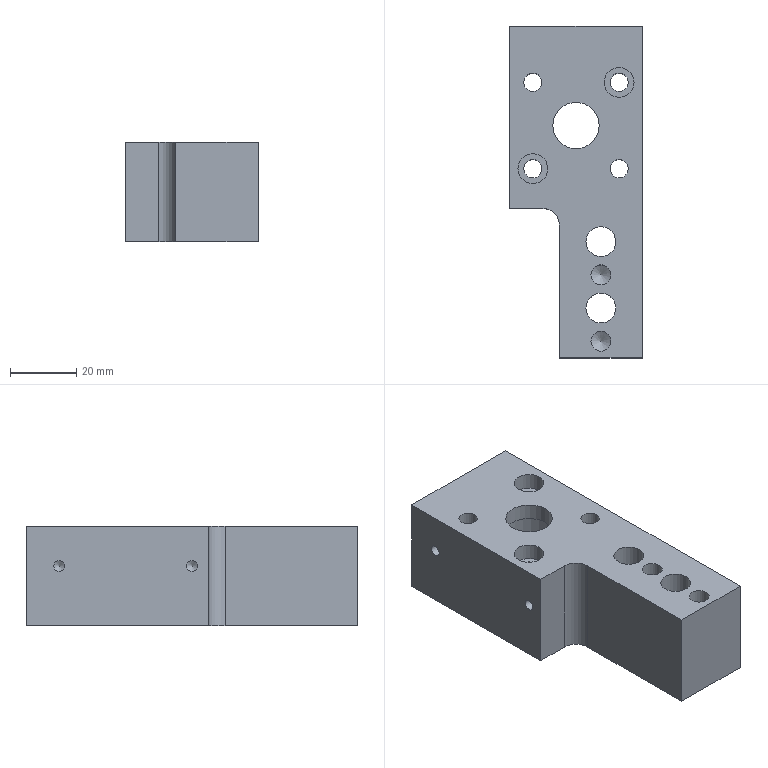Part | NX | features BREP 1 | 1 solid | 50 faces | box 40 x 100 x 30 mm | volume 78075 mm3 | cylinder 25 | plane 17 | cone 8 | commonest cylinder face diameters 10 x5 5.5 x4 6 x4 9 x4 3.3 x2 5 x2
STEP:
#1=CARTESIAN_POINT('',(-15.75,9.5,-9.6));
#2=VERTEX_POINT('',#1);
#3=CARTESIAN_POINT('',(-13.,9.5,-9.6));
#4=DIRECTION('',(0.,0.,-1.));
#5=DIRECTION('',(-1.,0.,0.));
#6=AXIS2_PLACEMENT_3D('',#3,#4,#5);
#7=CIRCLE('',#6,2.75);
#8=EDGE_CURVE('',#2,#2,#7,.T.);
#9=ORIENTED_EDGE('',*,*,#8,.T.);
#10=EDGE_LOOP('',(#9));
#11=FACE_BOUND('',#10,.T.);
#12=CARTESIAN_POINT('',(-10.25,9.5,10.));
#13=VERTEX_POINT('',#12);
#14=CARTESIAN_POINT('',(-13.,9.5,10.));
#15=DIRECTION('',(0.,0.,-1.));
#16=DIRECTION('',(1.,0.,0.));
#17=AXIS2_PLACEMENT_3D('',#14,#15,#16);
#18=CIRCLE('',#17,2.75);
#19=EDGE_CURVE('',#13,#13,#18,.T.);
#20=ORIENTED_EDGE('',*,*,#19,.F.);
#21=EDGE_LOOP('',(#20));
#22=FACE_BOUND('',#21,.T.);
#23=CARTESIAN_POINT('',(-13.,9.5,-15.));
#24=DIRECTION('',(0.,0.,-1.));
#25=DIRECTION('',(1.,0.,0.));
#26=AXIS2_PLACEMENT_3D('',#23,#24,#25);
#27=CYLINDRICAL_SURFACE('',#26,2.75);
#28=ADVANCED_FACE('',(#11,#22),#27,.F.);
#29=CARTESIAN_POINT('',(10.25,35.5,-9.6));
#30=VERTEX_POINT('',#29);
#31=CARTESIAN_POINT('',(13.,35.5,-9.6));
#32=DIRECTION('',(0.,0.,-1.));
#33=DIRECTION('',(-1.,0.,0.));
#34=AXIS2_PLACEMENT_3D('',#31,#32,#33);
#35=CIRCLE('',#34,2.75);
#36=EDGE_CURVE('',#30,#30,#35,.T.);
#37=ORIENTED_EDGE('',*,*,#36,.T.);
#38=EDGE_LOOP('',(#37));
#39=FACE_BOUND('',#38,.T.);
#40=CARTESIAN_POINT('',(15.75,35.5,10.));
#41=VERTEX_POINT('',#40);
#42=CARTESIAN_POINT('',(13.,35.5,10.));
#43=DIRECTION('',(0.,0.,-1.));
#44=DIRECTION('',(1.,0.,0.));
#45=AXIS2_PLACEMENT_3D('',#42,#43,#44);
#46=CIRCLE('',#45,2.75);
#47=EDGE_CURVE('',#41,#41,#46,.T.);
#48=ORIENTED_EDGE('',*,*,#47,.F.);
#49=EDGE_LOOP('',(#48));
#50=FACE_BOUND('',#49,.T.);
#51=CARTESIAN_POINT('',(13.,35.5,-15.));
#52=DIRECTION('',(0.,0.,-1.));
#53=DIRECTION('',(1.,0.,0.));
#54=AXIS2_PLACEMENT_3D('',#51,#52,#53);
#55=CYLINDRICAL_SURFACE('',#54,2.75);
#56=ADVANCED_FACE('',(#39,#50),#55,.F.);
#57=CARTESIAN_POINT('',(-10.5,22.5,-15.));
#58=VERTEX_POINT('',#57);
#59=CARTESIAN_POINT('',(0.,22.5,-15.));
#60=DIRECTION('',(0.,0.,-1.));
#61=DIRECTION('',(-1.,0.,0.));
#62=AXIS2_PLACEMENT_3D('',#59,#60,#61);
#63=CIRCLE('',#62,10.5);
#64=EDGE_CURVE('',#58,#58,#63,.T.);
#65=ORIENTED_EDGE('',*,*,#64,.T.);
#66=EDGE_LOOP('',(#65));
#67=FACE_BOUND('',#66,.T.);
#68=CARTESIAN_POINT('',(10.5,22.5,10.));
#69=VERTEX_POINT('',#68);
#70=CARTESIAN_POINT('',(0.,22.5,10.));
#71=DIRECTION('',(0.,0.,-1.));
#72=DIRECTION('',(1.,0.,0.));
#73=AXIS2_PLACEMENT_3D('',#70,#71,#72);
#74=CIRCLE('',#73,10.5);
#75=EDGE_CURVE('',#69,#69,#74,.T.);
#76=ORIENTED_EDGE('',*,*,#75,.F.);
#77=EDGE_LOOP('',(#76));
#78=FACE_BOUND('',#77,.T.);
#79=CARTESIAN_POINT('',(0.,22.5,-15.));
#80=DIRECTION('',(0.,0.,-1.));
#81=DIRECTION('',(1.,0.,0.));
#82=AXIS2_PLACEMENT_3D('',#79,#80,#81);
#83=CYLINDRICAL_SURFACE('',#82,10.5);
#84=ADVANCED_FACE('',(#67,#78),#83,.F.);
#85=CARTESIAN_POINT('',(20.,-47.5,15.));
#86=VERTEX_POINT('',#85);
#87=CARTESIAN_POINT('',(20.,52.5,15.));
#88=VERTEX_POINT('',#87);
#89=CARTESIAN_POINT('',(20.,-52.5,15.));
#90=DIRECTION('',(0.,1.,0.));
#91=VECTOR('',#90,1000.);
#92=LINE('',#89,#91);
#93=EDGE_CURVE('',#86,#88,#92,.T.);
#94=ORIENTED_EDGE('',*,*,#93,.F.);
#95=CARTESIAN_POINT('',(20.,-47.5,-15.));
#96=VERTEX_POINT('',#95);
#97=CARTESIAN_POINT('',(20.,-47.5,40.495));
#98=DIRECTION('',(0.,0.,-1.));
#99=VECTOR('',#98,1000.);
#100=LINE('',#97,#99);
#101=EDGE_CURVE('',#86,#96,#100,.T.);
#102=ORIENTED_EDGE('',*,*,#101,.T.);
#103=CARTESIAN_POINT('',(20.,52.5,-15.));
#104=VERTEX_POINT('',#103);
#105=CARTESIAN_POINT('',(20.,-52.5,-15.));
#106=DIRECTION('',(0.,1.,0.));
#107=VECTOR('',#106,1000.);
#108=LINE('',#105,#107);
#109=EDGE_CURVE('',#96,#104,#108,.T.);
#110=ORIENTED_EDGE('',*,*,#109,.T.);
#111=CARTESIAN_POINT('',(20.,52.5,15.));
#112=DIRECTION('',(0.,0.,-1.));
#113=VECTOR('',#112,1000.);
#114=LINE('',#111,#113);
#115=EDGE_CURVE('',#88,#104,#114,.T.);
#116=ORIENTED_EDGE('',*,*,#115,.F.);
#117=EDGE_LOOP('',(#94,#102,#110,#116));
#118=FACE_BOUND('',#117,.T.);
#119=CARTESIAN_POINT('',(20.,-52.5,15.));
#120=DIRECTION('',(-1.,0.,0.));
#121=DIRECTION('',(0.,0.,-1.));
#122=AXIS2_PLACEMENT_3D('',#119,#120,#121);
#123=PLANE('',#122);
#124=ADVANCED_FACE('',(#118),#123,.F.);
#125=CARTESIAN_POINT('',(-20.,52.5,-15.));
#126=VERTEX_POINT('',#125);
#127=CARTESIAN_POINT('',(-20.,52.5,-15.));
#128=DIRECTION('',(-1.,0.,0.));
#129=VECTOR('',#128,1000.);
#130=LINE('',#127,#129);
#131=EDGE_CURVE('',#104,#126,#130,.T.);
#132=ORIENTED_EDGE('',*,*,#131,.T.);
#133=CARTESIAN_POINT('',(-20.,52.5,15.));
#134=VERTEX_POINT('',#133);
#135=CARTESIAN_POINT('',(-20.,52.5,15.));
#136=DIRECTION('',(0.,0.,-1.));
#137=VECTOR('',#136,1000.);
#138=LINE('',#135,#137);
#139=EDGE_CURVE('',#134,#126,#138,.T.);
#140=ORIENTED_EDGE('',*,*,#139,.F.);
#141=CARTESIAN_POINT('',(-20.,52.5,15.));
#142=DIRECTION('',(-1.,0.,0.));
#143=VECTOR('',#142,1000.);
#144=LINE('',#141,#143);
#145=EDGE_CURVE('',#88,#134,#144,.T.);
#146=ORIENTED_EDGE('',*,*,#145,.F.);
#147=ORIENTED_EDGE('',*,*,#115,.T.);
#148=EDGE_LOOP('',(#132,#140,#146,#147));
#149=FACE_BOUND('',#148,.T.);
#150=CARTESIAN_POINT('',(-20.,52.5,15.));
#151=DIRECTION('',(0.,-1.,0.));
#152=DIRECTION('',(0.,0.,1.));
#153=AXIS2_PLACEMENT_3D('',#150,#151,#152);
#154=PLANE('',#153);
#155=ADVANCED_FACE('',(#149),#154,.F.);
#156=CARTESIAN_POINT('',(-20.,42.5,4.65));
#157=VERTEX_POINT('',#156);
#158=CARTESIAN_POINT('',(-20.,42.5,3.));
#159=DIRECTION('',(-1.,0.,0.));
#160=DIRECTION('',(0.,0.,1.));
#161=AXIS2_PLACEMENT_3D('',#158,#159,#160);
#162=CIRCLE('',#161,1.65);
#163=EDGE_CURVE('',#157,#157,#162,.T.);
#164=ORIENTED_EDGE('',*,*,#163,.F.);
#165=EDGE_LOOP('',(#164));
#166=FACE_BOUND('',#165,.T.);
#167=CARTESIAN_POINT('',(-20.,2.5,4.65));
#168=VERTEX_POINT('',#167);
#169=CARTESIAN_POINT('',(-20.,2.5,3.));
#170=DIRECTION('',(-1.,0.,0.));
#171=DIRECTION('',(0.,0.,1.));
#172=AXIS2_PLACEMENT_3D('',#169,#170,#171);
#173=CIRCLE('',#172,1.65);
#174=EDGE_CURVE('',#168,#168,#173,.T.);
#175=ORIENTED_EDGE('',*,*,#174,.F.);
#176=EDGE_LOOP('',(#175));
#177=FACE_BOUND('',#176,.T.);
#178=CARTESIAN_POINT('',(-20.,-2.5,-15.));
#179=VERTEX_POINT('',#178);
#180=CARTESIAN_POINT('',(-20.,-52.5,-15.));
#181=DIRECTION('',(0.,-1.,0.));
#182=VECTOR('',#181,1000.);
#183=LINE('',#180,#182);
#184=EDGE_CURVE('',#126,#179,#183,.T.);
#185=ORIENTED_EDGE('',*,*,#184,.T.);
#186=CARTESIAN_POINT('',(-20.,-2.5,15.));
#187=VERTEX_POINT('',#186);
#188=CARTESIAN_POINT('',(-20.,-2.5,67.202));
#189=DIRECTION('',(0.,0.,-1.));
#190=VECTOR('',#189,1000.);
#191=LINE('',#188,#190);
#192=EDGE_CURVE('',#187,#179,#191,.T.);
#193=ORIENTED_EDGE('',*,*,#192,.F.);
#194=CARTESIAN_POINT('',(-20.,-52.5,15.));
#195=DIRECTION('',(0.,-1.,0.));
#196=VECTOR('',#195,1000.);
#197=LINE('',#194,#196);
#198=EDGE_CURVE('',#134,#187,#197,.T.);
#199=ORIENTED_EDGE('',*,*,#198,.F.);
#200=ORIENTED_EDGE('',*,*,#139,.T.);
#201=EDGE_LOOP('',(#185,#193,#199,#200));
#202=FACE_BOUND('',#201,.T.);
#203=CARTESIAN_POINT('',(-20.,-52.5,15.));
#204=DIRECTION('',(1.,0.,0.));
#205=DIRECTION('',(0.,0.,1.));
#206=AXIS2_PLACEMENT_3D('',#203,#204,#205);
#207=PLANE('',#206);
#208=ADVANCED_FACE('',(#166,#177,#202),#207,.F.);
#209=CARTESIAN_POINT('',(17.5,35.5,15.));
#210=VERTEX_POINT('',#209);
#211=CARTESIAN_POINT('',(13.,35.5,15.));
#212=DIRECTION('',(0.,0.,1.));
#213=DIRECTION('',(1.,0.,0.));
#214=AXIS2_PLACEMENT_3D('',#211,#212,#213);
#215=CIRCLE('',#214,4.5);
#216=EDGE_CURVE('',#210,#210,#215,.T.);
#217=ORIENTED_EDGE('',*,*,#216,.F.);
#218=EDGE_LOOP('',(#217));
#219=FACE_BOUND('',#218,.T.);
#220=CARTESIAN_POINT('',(-8.5,9.5,15.));
#221=VERTEX_POINT('',#220);
#222=CARTESIAN_POINT('',(-13.,9.5,15.));
#223=DIRECTION('',(0.,0.,1.));
#224=DIRECTION('',(1.,0.,0.));
#225=AXIS2_PLACEMENT_3D('',#222,#223,#224);
#226=CIRCLE('',#225,4.5);
#227=EDGE_CURVE('',#221,#221,#226,.T.);
#228=ORIENTED_EDGE('',*,*,#227,.F.);
#229=EDGE_LOOP('',(#228));
#230=FACE_BOUND('',#229,.T.);
#231=CARTESIAN_POINT('',(10.25,9.5,15.));
#232=VERTEX_POINT('',#231);
#233=CARTESIAN_POINT('',(13.,9.5,15.));
#234=DIRECTION('',(0.,0.,-1.));
#235=DIRECTION('',(-1.,0.,0.));
#236=AXIS2_PLACEMENT_3D('',#233,#234,#235);
#237=CIRCLE('',#236,2.75);
#238=EDGE_CURVE('',#232,#232,#237,.T.);
#239=ORIENTED_EDGE('',*,*,#238,.T.);
#240=EDGE_LOOP('',(#239));
#241=FACE_BOUND('',#240,.T.);
#242=CARTESIAN_POINT('',(-15.75,35.5,15.));
#243=VERTEX_POINT('',#242);
#244=CARTESIAN_POINT('',(-13.,35.5,15.));
#245=DIRECTION('',(0.,0.,-1.));
#246=DIRECTION('',(-1.,0.,0.));
#247=AXIS2_PLACEMENT_3D('',#244,#245,#246);
#248=CIRCLE('',#247,2.75);
#249=EDGE_CURVE('',#243,#243,#248,.T.);
#250=ORIENTED_EDGE('',*,*,#249,.T.);
#251=EDGE_LOOP('',(#250));
#252=FACE_BOUND('',#251,.T.);
#253=CARTESIAN_POINT('',(3.,-12.5,15.));
#254=VERTEX_POINT('',#253);
#255=CARTESIAN_POINT('',(7.5,-12.5,15.));
#256=DIRECTION('',(0.,0.,-1.));
#257=DIRECTION('',(-1.,0.,0.));
#258=AXIS2_PLACEMENT_3D('',#255,#256,#257);
#259=CIRCLE('',#258,4.5);
#260=EDGE_CURVE('',#254,#254,#259,.T.);
#261=ORIENTED_EDGE('',*,*,#260,.T.);
#262=EDGE_LOOP('',(#261));
#263=FACE_BOUND('',#262,.T.);
#264=CARTESIAN_POINT('',(3.,-32.5,15.));
#265=VERTEX_POINT('',#264);
#266=CARTESIAN_POINT('',(7.5,-32.5,15.));
#267=DIRECTION('',(0.,0.,-1.));
#268=DIRECTION('',(-1.,0.,0.));
#269=AXIS2_PLACEMENT_3D('',#266,#267,#268);
#270=CIRCLE('',#269,4.5);
#271=EDGE_CURVE('',#265,#265,#270,.T.);
#272=ORIENTED_EDGE('',*,*,#271,.T.);
#273=EDGE_LOOP('',(#272));
#274=FACE_BOUND('',#273,.T.);
#275=CARTESIAN_POINT('',(10.5,-42.5,15.));
#276=VERTEX_POINT('',#275);
#277=CARTESIAN_POINT('',(7.5,-42.5,15.));
#278=DIRECTION('',(0.,0.,1.));
#279=DIRECTION('',(1.,0.,0.));
#280=AXIS2_PLACEMENT_3D('',#277,#278,#279);
#281=CIRCLE('',#280,3.);
#282=EDGE_CURVE('',#276,#276,#281,.T.);
#283=ORIENTED_EDGE('',*,*,#282,.F.);
#284=EDGE_LOOP('',(#283));
#285=FACE_BOUND('',#284,.T.);
#286=CARTESIAN_POINT('',(10.5,-22.5,15.));
#287=VERTEX_POINT('',#286);
#288=CARTESIAN_POINT('',(7.5,-22.5,15.));
#289=DIRECTION('',(0.,0.,1.));
#290=DIRECTION('',(1.,0.,0.));
#291=AXIS2_PLACEMENT_3D('',#288,#289,#290);
#292=CIRCLE('',#291,3.);
#293=EDGE_CURVE('',#287,#287,#292,.T.);
#294=ORIENTED_EDGE('',*,*,#293,.F.);
#295=EDGE_LOOP('',(#294));
#296=FACE_BOUND('',#295,.T.);
#297=CARTESIAN_POINT('',(-5.,-47.5,15.));
#298=VERTEX_POINT('',#297);
#299=CARTESIAN_POINT('',(-5.,-7.5,15.));
#300=VERTEX_POINT('',#299);
#301=CARTESIAN_POINT('',(-5.,-2.5,15.));
#302=DIRECTION('',(0.,1.,0.));
#303=VECTOR('',#302,1000.);
#304=LINE('',#301,#303);
#305=EDGE_CURVE('',#298,#300,#304,.T.);
#306=ORIENTED_EDGE('',*,*,#305,.F.);
#307=CARTESIAN_POINT('',(-5.,-47.5,15.));
#308=DIRECTION('',(-1.,0.,0.));
#309=VECTOR('',#308,1000.);
#310=LINE('',#307,#309);
#311=EDGE_CURVE('',#86,#298,#310,.T.);
#312=ORIENTED_EDGE('',*,*,#311,.F.);
#313=ORIENTED_EDGE('',*,*,#93,.T.);
#314=ORIENTED_EDGE('',*,*,#145,.T.);
#315=ORIENTED_EDGE('',*,*,#198,.T.);
#316=CARTESIAN_POINT('',(-10.,-2.5,15.));
#317=VERTEX_POINT('',#316);
#318=CARTESIAN_POINT('',(-20.,-2.5,15.));
#319=DIRECTION('',(-1.,0.,0.));
#320=VECTOR('',#319,1000.);
#321=LINE('',#318,#320);
#322=EDGE_CURVE('',#317,#187,#321,.T.);
#323=ORIENTED_EDGE('',*,*,#322,.F.);
#324=CARTESIAN_POINT('',(-10.,-7.5,15.));
#325=DIRECTION('',(0.,0.,-1.));
#326=DIRECTION('',(-1.,0.,0.));
#327=AXIS2_PLACEMENT_3D('',#324,#325,#326);
#328=CIRCLE('',#327,5.);
#329=EDGE_CURVE('',#317,#300,#328,.T.);
#330=ORIENTED_EDGE('',*,*,#329,.T.);
#331=EDGE_LOOP('',(#306,#312,#313,#314,#315,#323,#330));
#332=FACE_BOUND('',#331,.T.);
#333=CARTESIAN_POINT('',(7.,22.5,15.));
#334=VERTEX_POINT('',#333);
#335=CARTESIAN_POINT('',(0.,22.5,15.));
#336=DIRECTION('',(0.,0.,1.));
#337=DIRECTION('',(1.,0.,0.));
#338=AXIS2_PLACEMENT_3D('',#335,#336,#337);
#339=CIRCLE('',#338,7.);
#340=EDGE_CURVE('',#334,#334,#339,.T.);
#341=ORIENTED_EDGE('',*,*,#340,.F.);
#342=EDGE_LOOP('',(#341));
#343=FACE_BOUND('',#342,.T.);
#344=CARTESIAN_POINT('',(0.,0.,15.));
#345=DIRECTION('',(0.,0.,-1.));
#346=DIRECTION('',(1.,0.,0.));
#347=AXIS2_PLACEMENT_3D('',#344,#345,#346);
#348=PLANE('',#347);
#349=ADVANCED_FACE('',(#219,#230,#241,#252,#263,#274,#285,#296,#332,#343),#348,.F.);
#350=CARTESIAN_POINT('',(-5.,-47.5,-15.));
#351=VERTEX_POINT('',#350);
#352=CARTESIAN_POINT('',(-5.,-47.5,-15.));
#353=DIRECTION('',(1.,0.,0.));
#354=VECTOR('',#353,1000.);
#355=LINE('',#352,#354);
#356=EDGE_CURVE('',#351,#96,#355,.T.);
#357=ORIENTED_EDGE('',*,*,#356,.F.);
#358=CARTESIAN_POINT('',(-5.,-7.5,-15.));
#359=VERTEX_POINT('',#358);
#360=CARTESIAN_POINT('',(-5.,-2.5,-15.));
#361=DIRECTION('',(0.,-1.,0.));
#362=VECTOR('',#361,1000.);
#363=LINE('',#360,#362);
#364=EDGE_CURVE('',#359,#351,#363,.T.);
#365=ORIENTED_EDGE('',*,*,#364,.F.);
#366=CARTESIAN_POINT('',(-10.,-2.5,-15.));
#367=VERTEX_POINT('',#366);
#368=CARTESIAN_POINT('',(-10.,-7.5,-15.));
#369=DIRECTION('',(0.,0.,1.));
#370=DIRECTION('',(-1.,0.,0.));
#371=AXIS2_PLACEMENT_3D('',#368,#369,#370);
#372=CIRCLE('',#371,5.);
#373=EDGE_CURVE('',#359,#367,#372,.T.);
#374=ORIENTED_EDGE('',*,*,#373,.T.);
#375=CARTESIAN_POINT('',(-20.,-2.5,-15.));
#376=DIRECTION('',(1.,0.,0.));
#377=VECTOR('',#376,1000.);
#378=LINE('',#375,#377);
#379=EDGE_CURVE('',#179,#367,#378,.T.);
#380=ORIENTED_EDGE('',*,*,#379,.F.);
#381=ORIENTED_EDGE('',*,*,#184,.F.);
#382=ORIENTED_EDGE('',*,*,#131,.F.);
#383=ORIENTED_EDGE('',*,*,#109,.F.);
#384=EDGE_LOOP('',(#357,#365,#374,#380,#381,#382,#383));
#385=FACE_BOUND('',#384,.T.);
#386=CARTESIAN_POINT('',(-13.,45.,-15.));
#387=VERTEX_POINT('',#386);
#388=CARTESIAN_POINT('',(-10.,45.,-15.));
#389=DIRECTION('',(0.,0.,-1.));
#390=DIRECTION('',(-1.,0.,0.));
#391=AXIS2_PLACEMENT_3D('',#388,#389,#390);
#392=CIRCLE('',#391,3.);
#393=EDGE_CURVE('',#387,#387,#392,.T.);
#394=ORIENTED_EDGE('',*,*,#393,.F.);
#395=EDGE_LOOP('',(#394));
#396=FACE_BOUND('',#395,.T.);
#397=CARTESIAN_POINT('',(7.,0.,-15.));
#398=VERTEX_POINT('',#397);
#399=CARTESIAN_POINT('',(10.,0.,-15.));
#400=DIRECTION('',(0.,0.,-1.));
#401=DIRECTION('',(-1.,0.,0.));
#402=AXIS2_PLACEMENT_3D('',#399,#400,#401);
#403=CIRCLE('',#402,3.);
#404=EDGE_CURVE('',#398,#398,#403,.T.);
#405=ORIENTED_EDGE('',*,*,#404,.F.);
#406=EDGE_LOOP('',(#405));
#407=FACE_BOUND('',#406,.T.);
#408=CARTESIAN_POINT('',(-2.5,45.,-15.));
#409=VERTEX_POINT('',#408);
#410=CARTESIAN_POINT('',(0.,45.,-15.));
#411=DIRECTION('',(0.,0.,-1.));
#412=DIRECTION('',(-1.,0.,0.));
#413=AXIS2_PLACEMENT_3D('',#410,#411,#412);
#414=CIRCLE('',#413,2.5);
#415=EDGE_CURVE('',#409,#409,#414,.T.);
#416=ORIENTED_EDGE('',*,*,#415,.F.);
#417=EDGE_LOOP('',(#416));
#418=FACE_BOUND('',#417,.T.);
#419=CARTESIAN_POINT('',(-2.5,0.,-15.));
#420=VERTEX_POINT('',#419);
#421=CARTESIAN_POINT('',(0.,0.,-15.));
#422=DIRECTION('',(0.,0.,-1.));
#423=DIRECTION('',(-1.,0.,0.));
#424=AXIS2_PLACEMENT_3D('',#421,#422,#423);
#425=CIRCLE('',#424,2.5);
#426=EDGE_CURVE('',#420,#420,#425,.T.);
#427=ORIENTED_EDGE('',*,*,#426,.F.);
#428=EDGE_LOOP('',(#427));
#429=FACE_BOUND('',#428,.T.);
#430=CARTESIAN_POINT('',(8.,35.5,-15.));
#431=VERTEX_POINT('',#430);
#432=CARTESIAN_POINT('',(13.,35.5,-15.));
#433=DIRECTION('',(0.,0.,-1.));
#434=DIRECTION('',(-1.,0.,0.));
#435=AXIS2_PLACEMENT_3D('',#432,#433,#434);
#436=CIRCLE('',#435,5.);
#437=EDGE_CURVE('',#431,#431,#436,.T.);
#438=ORIENTED_EDGE('',*,*,#437,.F.);
#439=EDGE_LOOP('',(#438));
#440=FACE_BOUND('',#439,.T.);
#441=CARTESIAN_POINT('',(-18.,9.5,-15.));
#442=VERTEX_POINT('',#441);
#443=CARTESIAN_POINT('',(-13.,9.5,-15.));
#444=DIRECTION('',(0.,0.,-1.));
#445=DIRECTION('',(-1.,0.,0.));
#446=AXIS2_PLACEMENT_3D('',#443,#444,#445);
#447=CIRCLE('',#446,5.);
#448=EDGE_CURVE('',#442,#442,#447,.T.);
#449=ORIENTED_EDGE('',*,*,#448,.F.);
#450=EDGE_LOOP('',(#449));
#451=FACE_BOUND('',#450,.T.);
#452=CARTESIAN_POINT('',(8.,9.5,-15.));
#453=VERTEX_POINT('',#452);
#454=CARTESIAN_POINT('',(13.,9.5,-15.));
#455=DIRECTION('',(0.,0.,-1.));
#456=DIRECTION('',(-1.,0.,0.));
#457=AXIS2_PLACEMENT_3D('',#454,#455,#456);
#458=CIRCLE('',#457,5.);
#459=EDGE_CURVE('',#453,#453,#458,.T.);
#460=ORIENTED_EDGE('',*,*,#459,.F.);
#461=EDGE_LOOP('',(#460));
#462=FACE_BOUND('',#461,.T.);
#463=CARTESIAN_POINT('',(-18.,35.5,-15.));
#464=VERTEX_POINT('',#463);
#465=CARTESIAN_POINT('',(-13.,35.5,-15.));
#466=DIRECTION('',(0.,0.,-1.));
#467=DIRECTION('',(-1.,0.,0.));
#468=AXIS2_PLACEMENT_3D('',#465,#466,#467);
#469=CIRCLE('',#468,5.);
#470=EDGE_CURVE('',#464,#464,#469,.T.);
#471=ORIENTED_EDGE('',*,*,#470,.F.);
#472=EDGE_LOOP('',(#471));
#473=FACE_BOUND('',#472,.T.);
#474=CARTESIAN_POINT('',(0.,-12.5,-15.));
#475=VERTEX_POINT('',#474);
#476=CARTESIAN_POINT('',(7.5,-12.5,-15.));
#477=DIRECTION('',(0.,0.,-1.));
#478=DIRECTION('',(-1.,0.,0.));
#479=AXIS2_PLACEMENT_3D('',#476,#477,#478);
#480=CIRCLE('',#479,7.5);
#481=EDGE_CURVE('',#475,#475,#480,.T.);
#482=ORIENTED_EDGE('',*,*,#481,.F.);
#483=EDGE_LOOP('',(#482));
#484=FACE_BOUND('',#483,.T.);
#485=CARTESIAN_POINT('',(0.,-32.5,-15.));
#486=VERTEX_POINT('',#485);
#487=CARTESIAN_POINT('',(7.5,-32.5,-15.));
#488=DIRECTION('',(0.,0.,-1.));
#489=DIRECTION('',(-1.,0.,0.));
#490=AXIS2_PLACEMENT_3D('',#487,#488,#489);
#491=CIRCLE('',#490,7.5);
#492=EDGE_CURVE('',#486,#486,#491,.T.);
#493=ORIENTED_EDGE('',*,*,#492,.F.);
#494=EDGE_LOOP('',(#493));
#495=FACE_BOUND('',#494,.T.);
#496=ORIENTED_EDGE('',*,*,#64,.F.);
#497=EDGE_LOOP('',(#496));
#498=FACE_BOUND('',#497,.T.);
#499=CARTESIAN_POINT('',(0.,0.,-15.));
#500=DIRECTION('',(0.,0.,-1.));
#501=DIRECTION('',(1.,0.,0.));
#502=AXIS2_PLACEMENT_3D('',#499,#500,#501);
#503=PLANE('',#502);
#504=ADVANCED_FACE('',(#385,#396,#407,#418,#429,#440,#451,#462,#473,#484,#495,#498),#503,.T.);
#505=CARTESIAN_POINT('',(7.,22.5,10.));
#506=VERTEX_POINT('',#505);
#507=CARTESIAN_POINT('',(0.,22.5,10.));
#508=DIRECTION('',(0.,0.,1.));
#509=DIRECTION('',(1.,0.,0.));
#510=AXIS2_PLACEMENT_3D('',#507,#508,#509);
#511=CIRCLE('',#510,7.);
#512=EDGE_CURVE('',#506,#506,#511,.T.);
#513=ORIENTED_EDGE('',*,*,#512,.T.);
#514=EDGE_LOOP('',(#513));
#515=FACE_BOUND('',#514,.T.);
#516=ORIENTED_EDGE('',*,*,#75,.T.);
#517=EDGE_LOOP('',(#516));
#518=FACE_BOUND('',#517,.T.);
#519=CARTESIAN_POINT('',(0.,22.5,10.));
#520=DIRECTION('',(0.,0.,1.));
#521=DIRECTION('',(-1.,0.,0.));
#522=AXIS2_PLACEMENT_3D('',#519,#520,#521);
#523=PLANE('',#522);
#524=ADVANCED_FACE('',(#515,#518),#523,.F.);
#525=ORIENTED_EDGE('',*,*,#512,.F.);
#526=EDGE_LOOP('',(#525));
#527=FACE_BOUND('',#526,.T.);
#528=ORIENTED_EDGE('',*,*,#340,.T.);
#529=EDGE_LOOP('',(#528));
#530=FACE_BOUND('',#529,.T.);
#531=CARTESIAN_POINT('',(0.,22.5,10.));
#532=DIRECTION('',(0.,0.,1.));
#533=DIRECTION('',(-1.,0.,0.));
#534=AXIS2_PLACEMENT_3D('',#531,#532,#533);
#535=CYLINDRICAL_SURFACE('',#534,7.);
#536=ADVANCED_FACE('',(#527,#530),#535,.F.);
#537=ORIENTED_EDGE('',*,*,#364,.T.);
#538=CARTESIAN_POINT('',(-5.,-47.5,40.495));
#539=DIRECTION('',(0.,0.,-1.));
#540=VECTOR('',#539,1000.);
#541=LINE('',#538,#540);
#542=EDGE_CURVE('',#298,#351,#541,.T.);
#543=ORIENTED_EDGE('',*,*,#542,.F.);
#544=ORIENTED_EDGE('',*,*,#305,.T.);
#545=CARTESIAN_POINT('',(-5.,-7.5,-15.));
#546=DIRECTION('',(0.,0.,-1.));
#547=VECTOR('',#546,1000.);
#548=LINE('',#545,#547);
#549=EDGE_CURVE('',#300,#359,#548,.T.);
#550=ORIENTED_EDGE('',*,*,#549,.T.);
#551=EDGE_LOOP('',(#537,#543,#544,#550));
#552=FACE_BOUND('',#551,.T.);
#553=CARTESIAN_POINT('',(-5.,-2.5,67.202));
#554=DIRECTION('',(1.,0.,0.));
#555=DIRECTION('',(0.,-1.,0.));
#556=AXIS2_PLACEMENT_3D('',#553,#554,#555);
#557=PLANE('',#556);
#558=ADVANCED_FACE('',(#552),#557,.F.);
#559=ORIENTED_EDGE('',*,*,#379,.T.);
#560=CARTESIAN_POINT('',(-10.,-2.5,15.));
#561=DIRECTION('',(0.,0.,1.));
#562=VECTOR('',#561,1000.);
#563=LINE('',#560,#562);
#564=EDGE_CURVE('',#367,#317,#563,.T.);
#565=ORIENTED_EDGE('',*,*,#564,.T.);
#566=ORIENTED_EDGE('',*,*,#322,.T.);
#567=ORIENTED_EDGE('',*,*,#192,.T.);
#568=EDGE_LOOP('',(#559,#565,#566,#567));
#569=FACE_BOUND('',#568,.T.);
#570=CARTESIAN_POINT('',(-20.,-2.5,67.202));
#571=DIRECTION('',(0.,1.,0.));
#572=DIRECTION('',(0.,0.,-1.));
#573=AXIS2_PLACEMENT_3D('',#570,#571,#572);
#574=PLANE('',#573);
#575=ADVANCED_FACE('',(#569),#574,.F.);
#576=CARTESIAN_POINT('',(7.5,-22.5,1.197));
#577=VERTEX_POINT('',#576);
#578=VERTEX_LOOP('',#577);
#579=FACE_BOUND('',#578,.T.);
#580=CARTESIAN_POINT('',(10.5,-22.5,3.));
#581=VERTEX_POINT('',#580);
#582=CARTESIAN_POINT('',(7.5,-22.5,3.));
#583=DIRECTION('',(0.,0.,1.));
#584=DIRECTION('',(1.,0.,0.));
#585=AXIS2_PLACEMENT_3D('',#582,#583,#584);
#586=CIRCLE('',#585,3.);
#587=EDGE_CURVE('',#581,#581,#586,.T.);
#588=ORIENTED_EDGE('',*,*,#587,.T.);
#589=EDGE_LOOP('',(#588));
#590=FACE_BOUND('',#589,.T.);
#591=CARTESIAN_POINT('',(7.5,-22.5,3.));
#592=DIRECTION('',(0.,0.,1.));
#593=DIRECTION('',(-1.,0.,0.));
#594=AXIS2_PLACEMENT_3D('',#591,#592,#593);
#595=CONICAL_SURFACE('',#594,3.,1.03);
#596=ADVANCED_FACE('',(#579,#590),#595,.F.);
#597=ORIENTED_EDGE('',*,*,#587,.F.);
#598=EDGE_LOOP('',(#597));
#599=FACE_BOUND('',#598,.T.);
#600=ORIENTED_EDGE('',*,*,#293,.T.);
#601=EDGE_LOOP('',(#600));
#602=FACE_BOUND('',#601,.T.);
#603=CARTESIAN_POINT('',(7.5,-22.5,15.));
#604=DIRECTION('',(0.,0.,1.));
#605=DIRECTION('',(-1.,0.,0.));
#606=AXIS2_PLACEMENT_3D('',#603,#604,#605);
#607=CYLINDRICAL_SURFACE('',#606,3.);
#608=ADVANCED_FACE('',(#599,#602),#607,.F.);
#609=CARTESIAN_POINT('',(7.5,-42.5,1.197));
#610=VERTEX_POINT('',#609);
#611=VERTEX_LOOP('',#610);
#612=FACE_BOUND('',#611,.T.);
#613=CARTESIAN_POINT('',(10.5,-42.5,3.));
#614=VERTEX_POINT('',#613);
#615=CARTESIAN_POINT('',(7.5,-42.5,3.));
#616=DIRECTION('',(0.,0.,1.));
#617=DIRECTION('',(1.,0.,0.));
#618=AXIS2_PLACEMENT_3D('',#615,#616,#617);
#619=CIRCLE('',#618,3.);
#620=EDGE_CURVE('',#614,#614,#619,.T.);
#621=ORIENTED_EDGE('',*,*,#620,.T.);
#622=EDGE_LOOP('',(#621));
#623=FACE_BOUND('',#622,.T.);
#624=CARTESIAN_POINT('',(7.5,-42.5,3.));
#625=DIRECTION('',(0.,0.,1.));
#626=DIRECTION('',(-1.,0.,0.));
#627=AXIS2_PLACEMENT_3D('',#624,#625,#626);
#628=CONICAL_SURFACE('',#627,3.,1.03);
#629=ADVANCED_FACE('',(#612,#623),#628,.F.);
#630=ORIENTED_EDGE('',*,*,#620,.F.);
#631=EDGE_LOOP('',(#630));
#632=FACE_BOUND('',#631,.T.);
#633=ORIENTED_EDGE('',*,*,#282,.T.);
#634=EDGE_LOOP('',(#633));
#635=FACE_BOUND('',#634,.T.);
#636=CARTESIAN_POINT('',(7.5,-42.5,15.));
#637=DIRECTION('',(0.,0.,1.));
#638=DIRECTION('',(-1.,0.,0.));
#639=AXIS2_PLACEMENT_3D('',#636,#637,#638);
#640=CYLINDRICAL_SURFACE('',#639,3.);
#641=ADVANCED_FACE('',(#632,#635),#640,.F.);
#642=ORIENTED_EDGE('',*,*,#271,.F.);
#643=EDGE_LOOP('',(#642));
#644=FACE_BOUND('',#643,.T.);
#645=CARTESIAN_POINT('',(3.,-32.5,-6.4));
#646=VERTEX_POINT('',#645);
#647=CARTESIAN_POINT('',(7.5,-32.5,-6.4));
#648=DIRECTION('',(0.,0.,-1.));
#649=DIRECTION('',(-1.,0.,0.));
#650=AXIS2_PLACEMENT_3D('',#647,#648,#649);
#651=CIRCLE('',#650,4.5);
#652=EDGE_CURVE('',#646,#646,#651,.T.);
#653=ORIENTED_EDGE('',*,*,#652,.T.);
#654=EDGE_LOOP('',(#653));
#655=FACE_BOUND('',#654,.T.);
#656=CARTESIAN_POINT('',(7.5,-32.5,-15.));
#657=DIRECTION('',(0.,0.,-1.));
#658=DIRECTION('',(1.,0.,0.));
#659=AXIS2_PLACEMENT_3D('',#656,#657,#658);
#660=CYLINDRICAL_SURFACE('',#659,4.5);
#661=ADVANCED_FACE('',(#644,#655),#660,.F.);
#662=ORIENTED_EDGE('',*,*,#652,.F.);
#663=EDGE_LOOP('',(#662));
#664=FACE_BOUND('',#663,.T.);
#665=CARTESIAN_POINT('',(0.,-32.5,-6.4));
#666=VERTEX_POINT('',#665);
#667=CARTESIAN_POINT('',(7.5,-32.5,-6.4));
#668=DIRECTION('',(0.,0.,-1.));
#669=DIRECTION('',(-1.,0.,0.));
#670=AXIS2_PLACEMENT_3D('',#667,#668,#669);
#671=CIRCLE('',#670,7.5);
#672=EDGE_CURVE('',#666,#666,#671,.T.);
#673=ORIENTED_EDGE('',*,*,#672,.T.);
#674=EDGE_LOOP('',(#673));
#675=FACE_BOUND('',#674,.T.);
#676=CARTESIAN_POINT('',(12.,-32.5,-6.4));
#677=DIRECTION('',(0.,0.,1.));
#678=DIRECTION('',(-1.,0.,0.));
#679=AXIS2_PLACEMENT_3D('',#676,#677,#678);
#680=PLANE('',#679);
#681=ADVANCED_FACE('',(#664,#675),#680,.F.);
#682=ORIENTED_EDGE('',*,*,#672,.F.);
#683=EDGE_LOOP('',(#682));
#684=FACE_BOUND('',#683,.T.);
#685=ORIENTED_EDGE('',*,*,#492,.T.);
#686=EDGE_LOOP('',(#685));
#687=FACE_BOUND('',#686,.T.);
#688=CARTESIAN_POINT('',(7.5,-32.5,-15.));
#689=DIRECTION('',(0.,0.,-1.));
#690=DIRECTION('',(1.,0.,0.));
#691=AXIS2_PLACEMENT_3D('',#688,#689,#690);
#692=CYLINDRICAL_SURFACE('',#691,7.5);
#693=ADVANCED_FACE('',(#684,#687),#692,.F.);
#694=ORIENTED_EDGE('',*,*,#260,.F.);
#695=EDGE_LOOP('',(#694));
#696=FACE_BOUND('',#695,.T.);
#697=CARTESIAN_POINT('',(3.,-12.5,-6.4));
#698=VERTEX_POINT('',#697);
#699=CARTESIAN_POINT('',(7.5,-12.5,-6.4));
#700=DIRECTION('',(0.,0.,-1.));
#701=DIRECTION('',(-1.,0.,0.));
#702=AXIS2_PLACEMENT_3D('',#699,#700,#701);
#703=CIRCLE('',#702,4.5);
#704=EDGE_CURVE('',#698,#698,#703,.T.);
#705=ORIENTED_EDGE('',*,*,#704,.T.);
#706=EDGE_LOOP('',(#705));
#707=FACE_BOUND('',#706,.T.);
#708=CARTESIAN_POINT('',(7.5,-12.5,-15.));
#709=DIRECTION('',(0.,0.,-1.));
#710=DIRECTION('',(1.,0.,0.));
#711=AXIS2_PLACEMENT_3D('',#708,#709,#710);
#712=CYLINDRICAL_SURFACE('',#711,4.5);
#713=ADVANCED_FACE('',(#696,#707),#712,.F.);
#714=ORIENTED_EDGE('',*,*,#704,.F.);
#715=EDGE_LOOP('',(#714));
#716=FACE_BOUND('',#715,.T.);
#717=CARTESIAN_POINT('',(0.,-12.5,-6.4));
#718=VERTEX_POINT('',#717);
#719=CARTESIAN_POINT('',(7.5,-12.5,-6.4));
#720=DIRECTION('',(0.,0.,-1.));
#721=DIRECTION('',(-1.,0.,0.));
#722=AXIS2_PLACEMENT_3D('',#719,#720,#721);
#723=CIRCLE('',#722,7.5);
#724=EDGE_CURVE('',#718,#718,#723,.T.);
#725=ORIENTED_EDGE('',*,*,#724,.T.);
#726=EDGE_LOOP('',(#725));
#727=FACE_BOUND('',#726,.T.);
#728=CARTESIAN_POINT('',(12.,-12.5,-6.4));
#729=DIRECTION('',(0.,0.,1.));
#730=DIRECTION('',(-1.,0.,0.));
#731=AXIS2_PLACEMENT_3D('',#728,#729,#730);
#732=PLANE('',#731);
#733=ADVANCED_FACE('',(#716,#727),#732,.F.);
#734=ORIENTED_EDGE('',*,*,#724,.F.);
#735=EDGE_LOOP('',(#734));
#736=FACE_BOUND('',#735,.T.);
#737=ORIENTED_EDGE('',*,*,#481,.T.);
#738=EDGE_LOOP('',(#737));
#739=FACE_BOUND('',#738,.T.);
#740=CARTESIAN_POINT('',(7.5,-12.5,-15.));
#741=DIRECTION('',(0.,0.,-1.));
#742=DIRECTION('',(1.,0.,0.));
#743=AXIS2_PLACEMENT_3D('',#740,#741,#742);
#744=CYLINDRICAL_SURFACE('',#743,7.5);
#745=ADVANCED_FACE('',(#736,#739),#744,.F.);
#746=ORIENTED_EDGE('',*,*,#329,.F.);
#747=ORIENTED_EDGE('',*,*,#564,.F.);
#748=ORIENTED_EDGE('',*,*,#373,.F.);
#749=ORIENTED_EDGE('',*,*,#549,.F.);
#750=EDGE_LOOP('',(#746,#747,#748,#749));
#751=FACE_BOUND('',#750,.T.);
#752=CARTESIAN_POINT('',(-10.,-7.5,67.202));
#753=DIRECTION('',(0.,0.,1.));
#754=DIRECTION('',(-1.,0.,0.));
#755=AXIS2_PLACEMENT_3D('',#752,#753,#754);
#756=CYLINDRICAL_SURFACE('',#755,5.);
#757=ADVANCED_FACE('',(#751),#756,.F.);
#758=ORIENTED_EDGE('',*,*,#249,.F.);
#759=EDGE_LOOP('',(#758));
#760=FACE_BOUND('',#759,.T.);
#761=CARTESIAN_POINT('',(-15.75,35.5,-9.6));
#762=VERTEX_POINT('',#761);
#763=CARTESIAN_POINT('',(-13.,35.5,-9.6));
#764=DIRECTION('',(0.,0.,-1.));
#765=DIRECTION('',(-1.,0.,0.));
#766=AXIS2_PLACEMENT_3D('',#763,#764,#765);
#767=CIRCLE('',#766,2.75);
#768=EDGE_CURVE('',#762,#762,#767,.T.);
#769=ORIENTED_EDGE('',*,*,#768,.T.);
#770=EDGE_LOOP('',(#769));
#771=FACE_BOUND('',#770,.T.);
#772=CARTESIAN_POINT('',(-13.,35.5,-15.));
#773=DIRECTION('',(0.,0.,-1.));
#774=DIRECTION('',(1.,0.,0.));
#775=AXIS2_PLACEMENT_3D('',#772,#773,#774);
#776=CYLINDRICAL_SURFACE('',#775,2.75);
#777=ADVANCED_FACE('',(#760,#771),#776,.F.);
#778=ORIENTED_EDGE('',*,*,#768,.F.);
#779=EDGE_LOOP('',(#778));
#780=FACE_BOUND('',#779,.T.);
#781=CARTESIAN_POINT('',(-18.,35.5,-9.6));
#782=VERTEX_POINT('',#781);
#783=CARTESIAN_POINT('',(-13.,35.5,-9.6));
#784=DIRECTION('',(0.,0.,-1.));
#785=DIRECTION('',(-1.,0.,0.));
#786=AXIS2_PLACEMENT_3D('',#783,#784,#785);
#787=CIRCLE('',#786,5.);
#788=EDGE_CURVE('',#782,#782,#787,.T.);
#789=ORIENTED_EDGE('',*,*,#788,.T.);
#790=EDGE_LOOP('',(#789));
#791=FACE_BOUND('',#790,.T.);
#792=CARTESIAN_POINT('',(-10.25,35.5,-9.6));
#793=DIRECTION('',(0.,0.,1.));
#794=DIRECTION('',(-1.,0.,0.));
#795=AXIS2_PLACEMENT_3D('',#792,#793,#794);
#796=PLANE('',#795);
#797=ADVANCED_FACE('',(#780,#791),#796,.F.);
#798=ORIENTED_EDGE('',*,*,#788,.F.);
#799=EDGE_LOOP('',(#798));
#800=FACE_BOUND('',#799,.T.);
#801=ORIENTED_EDGE('',*,*,#470,.T.);
#802=EDGE_LOOP('',(#801));
#803=FACE_BOUND('',#802,.T.);
#804=CARTESIAN_POINT('',(-13.,35.5,-15.));
#805=DIRECTION('',(0.,0.,-1.));
#806=DIRECTION('',(1.,0.,0.));
#807=AXIS2_PLACEMENT_3D('',#804,#805,#806);
#808=CYLINDRICAL_SURFACE('',#807,5.);
#809=ADVANCED_FACE('',(#800,#803),#808,.F.);
#810=ORIENTED_EDGE('',*,*,#238,.F.);
#811=EDGE_LOOP('',(#810));
#812=FACE_BOUND('',#811,.T.);
#813=CARTESIAN_POINT('',(10.25,9.5,-9.6));
#814=VERTEX_POINT('',#813);
#815=CARTESIAN_POINT('',(13.,9.5,-9.6));
#816=DIRECTION('',(0.,0.,-1.));
#817=DIRECTION('',(-1.,0.,0.));
#818=AXIS2_PLACEMENT_3D('',#815,#816,#817);
#819=CIRCLE('',#818,2.75);
#820=EDGE_CURVE('',#814,#814,#819,.T.);
#821=ORIENTED_EDGE('',*,*,#820,.T.);
#822=EDGE_LOOP('',(#821));
#823=FACE_BOUND('',#822,.T.);
#824=CARTESIAN_POINT('',(13.,9.5,-15.));
#825=DIRECTION('',(0.,0.,-1.));
#826=DIRECTION('',(1.,0.,0.));
#827=AXIS2_PLACEMENT_3D('',#824,#825,#826);
#828=CYLINDRICAL_SURFACE('',#827,2.75);
#829=ADVANCED_FACE('',(#812,#823),#828,.F.);
#830=ORIENTED_EDGE('',*,*,#820,.F.);
#831=EDGE_LOOP('',(#830));
#832=FACE_BOUND('',#831,.T.);
#833=CARTESIAN_POINT('',(8.,9.5,-9.6));
#834=VERTEX_POINT('',#833);
#835=CARTESIAN_POINT('',(13.,9.5,-9.6));
#836=DIRECTION('',(0.,0.,-1.));
#837=DIRECTION('',(-1.,0.,0.));
#838=AXIS2_PLACEMENT_3D('',#835,#836,#837);
#839=CIRCLE('',#838,5.);
#840=EDGE_CURVE('',#834,#834,#839,.T.);
#841=ORIENTED_EDGE('',*,*,#840,.T.);
#842=EDGE_LOOP('',(#841));
#843=FACE_BOUND('',#842,.T.);
#844=CARTESIAN_POINT('',(15.75,9.5,-9.6));
#845=DIRECTION('',(0.,0.,1.));
#846=DIRECTION('',(-1.,0.,0.));
#847=AXIS2_PLACEMENT_3D('',#844,#845,#846);
#848=PLANE('',#847);
#849=ADVANCED_FACE('',(#832,#843),#848,.F.);
#850=ORIENTED_EDGE('',*,*,#840,.F.);
#851=EDGE_LOOP('',(#850));
#852=FACE_BOUND('',#851,.T.);
#853=ORIENTED_EDGE('',*,*,#459,.T.);
#854=EDGE_LOOP('',(#853));
#855=FACE_BOUND('',#854,.T.);
#856=CARTESIAN_POINT('',(13.,9.5,-15.));
#857=DIRECTION('',(0.,0.,-1.));
#858=DIRECTION('',(1.,0.,0.));
#859=AXIS2_PLACEMENT_3D('',#856,#857,#858);
#860=CYLINDRICAL_SURFACE('',#859,5.);
#861=ADVANCED_FACE('',(#852,#855),#860,.F.);
#862=ORIENTED_EDGE('',*,*,#8,.F.);
#863=EDGE_LOOP('',(#862));
#864=FACE_BOUND('',#863,.T.);
#865=CARTESIAN_POINT('',(-18.,9.5,-9.6));
#866=VERTEX_POINT('',#865);
#867=CARTESIAN_POINT('',(-13.,9.5,-9.6));
#868=DIRECTION('',(0.,0.,-1.));
#869=DIRECTION('',(-1.,0.,0.));
#870=AXIS2_PLACEMENT_3D('',#867,#868,#869);
#871=CIRCLE('',#870,5.);
#872=EDGE_CURVE('',#866,#866,#871,.T.);
#873=ORIENTED_EDGE('',*,*,#872,.T.);
#874=EDGE_LOOP('',(#873));
#875=FACE_BOUND('',#874,.T.);
#876=CARTESIAN_POINT('',(-10.25,9.5,-9.6));
#877=DIRECTION('',(0.,0.,1.));
#878=DIRECTION('',(-1.,0.,0.));
#879=AXIS2_PLACEMENT_3D('',#876,#877,#878);
#880=PLANE('',#879);
#881=ADVANCED_FACE('',(#864,#875),#880,.F.);
#882=ORIENTED_EDGE('',*,*,#872,.F.);
#883=EDGE_LOOP('',(#882));
#884=FACE_BOUND('',#883,.T.);
#885=ORIENTED_EDGE('',*,*,#448,.T.);
#886=EDGE_LOOP('',(#885));
#887=FACE_BOUND('',#886,.T.);
#888=CARTESIAN_POINT('',(-13.,9.5,-15.));
#889=DIRECTION('',(0.,0.,-1.));
#890=DIRECTION('',(1.,0.,0.));
#891=AXIS2_PLACEMENT_3D('',#888,#889,#890);
#892=CYLINDRICAL_SURFACE('',#891,5.);
#893=ADVANCED_FACE('',(#884,#887),#892,.F.);
#894=ORIENTED_EDGE('',*,*,#36,.F.);
#895=EDGE_LOOP('',(#894));
#896=FACE_BOUND('',#895,.T.);
#897=CARTESIAN_POINT('',(8.,35.5,-9.6));
#898=VERTEX_POINT('',#897);
#899=CARTESIAN_POINT('',(13.,35.5,-9.6));
#900=DIRECTION('',(0.,0.,-1.));
#901=DIRECTION('',(-1.,0.,0.));
#902=AXIS2_PLACEMENT_3D('',#899,#900,#901);
#903=CIRCLE('',#902,5.);
#904=EDGE_CURVE('',#898,#898,#903,.T.);
#905=ORIENTED_EDGE('',*,*,#904,.T.);
#906=EDGE_LOOP('',(#905));
#907=FACE_BOUND('',#906,.T.);
#908=CARTESIAN_POINT('',(15.75,35.5,-9.6));
#909=DIRECTION('',(0.,0.,1.));
#910=DIRECTION('',(-1.,0.,0.));
#911=AXIS2_PLACEMENT_3D('',#908,#909,#910);
#912=PLANE('',#911);
#913=ADVANCED_FACE('',(#896,#907),#912,.F.);
#914=ORIENTED_EDGE('',*,*,#904,.F.);
#915=EDGE_LOOP('',(#914));
#916=FACE_BOUND('',#915,.T.);
#917=ORIENTED_EDGE('',*,*,#437,.T.);
#918=EDGE_LOOP('',(#917));
#919=FACE_BOUND('',#918,.T.);
#920=CARTESIAN_POINT('',(13.,35.5,-15.));
#921=DIRECTION('',(0.,0.,-1.));
#922=DIRECTION('',(1.,0.,0.));
#923=AXIS2_PLACEMENT_3D('',#920,#921,#922);
#924=CYLINDRICAL_SURFACE('',#923,5.);
#925=ADVANCED_FACE('',(#916,#919),#924,.F.);
#926=CARTESIAN_POINT('',(17.5,35.5,10.));
#927=VERTEX_POINT('',#926);
#928=CARTESIAN_POINT('',(13.,35.5,10.));
#929=DIRECTION('',(0.,0.,1.));
#930=DIRECTION('',(1.,0.,0.));
#931=AXIS2_PLACEMENT_3D('',#928,#929,#930);
#932=CIRCLE('',#931,4.5);
#933=EDGE_CURVE('',#927,#927,#932,.T.);
#934=ORIENTED_EDGE('',*,*,#933,.T.);
#935=EDGE_LOOP('',(#934));
#936=FACE_BOUND('',#935,.T.);
#937=ORIENTED_EDGE('',*,*,#47,.T.);
#938=EDGE_LOOP('',(#937));
#939=FACE_BOUND('',#938,.T.);
#940=CARTESIAN_POINT('',(13.,35.5,10.));
#941=DIRECTION('',(0.,0.,1.));
#942=DIRECTION('',(-1.,0.,0.));
#943=AXIS2_PLACEMENT_3D('',#940,#941,#942);
#944=PLANE('',#943);
#945=ADVANCED_FACE('',(#936,#939),#944,.T.);
#946=ORIENTED_EDGE('',*,*,#933,.F.);
#947=EDGE_LOOP('',(#946));
#948=FACE_BOUND('',#947,.T.);
#949=ORIENTED_EDGE('',*,*,#216,.T.);
#950=EDGE_LOOP('',(#949));
#951=FACE_BOUND('',#950,.T.);
#952=CARTESIAN_POINT('',(13.,35.5,10.));
#953=DIRECTION('',(0.,0.,1.));
#954=DIRECTION('',(-1.,0.,0.));
#955=AXIS2_PLACEMENT_3D('',#952,#953,#954);
#956=CYLINDRICAL_SURFACE('',#955,4.5);
#957=ADVANCED_FACE('',(#948,#951),#956,.F.);
#958=CARTESIAN_POINT('',(-8.5,9.5,10.));
#959=VERTEX_POINT('',#958);
#960=CARTESIAN_POINT('',(-13.,9.5,10.));
#961=DIRECTION('',(0.,0.,1.));
#962=DIRECTION('',(1.,0.,0.));
#963=AXIS2_PLACEMENT_3D('',#960,#961,#962);
#964=CIRCLE('',#963,4.5);
#965=EDGE_CURVE('',#959,#959,#964,.T.);
#966=ORIENTED_EDGE('',*,*,#965,.T.);
#967=EDGE_LOOP('',(#966));
#968=FACE_BOUND('',#967,.T.);
#969=ORIENTED_EDGE('',*,*,#19,.T.);
#970=EDGE_LOOP('',(#969));
#971=FACE_BOUND('',#970,.T.);
#972=CARTESIAN_POINT('',(-13.,9.5,10.));
#973=DIRECTION('',(0.,0.,1.));
#974=DIRECTION('',(-1.,0.,0.));
#975=AXIS2_PLACEMENT_3D('',#972,#973,#974);
#976=PLANE('',#975);
#977=ADVANCED_FACE('',(#968,#971),#976,.T.);
#978=ORIENTED_EDGE('',*,*,#965,.F.);
#979=EDGE_LOOP('',(#978));
#980=FACE_BOUND('',#979,.T.);
#981=ORIENTED_EDGE('',*,*,#227,.T.);
#982=EDGE_LOOP('',(#981));
#983=FACE_BOUND('',#982,.T.);
#984=CARTESIAN_POINT('',(-13.,9.5,10.));
#985=DIRECTION('',(0.,0.,1.));
#986=DIRECTION('',(-1.,0.,0.));
#987=AXIS2_PLACEMENT_3D('',#984,#985,#986);
#988=CYLINDRICAL_SURFACE('',#987,4.5);
#989=ADVANCED_FACE('',(#980,#983),#988,.F.);
#990=CARTESIAN_POINT('',(0.,0.,1.502));
#991=VERTEX_POINT('',#990);
#992=VERTEX_LOOP('',#991);
#993=FACE_BOUND('',#992,.T.);
#994=CARTESIAN_POINT('',(-2.5,0.,0.));
#995=VERTEX_POINT('',#994);
#996=CARTESIAN_POINT('',(0.,0.,0.));
#997=DIRECTION('',(0.,0.,-1.));
#998=DIRECTION('',(-1.,0.,0.));
#999=AXIS2_PLACEMENT_3D('',#996,#997,#998);
#1000=CIRCLE('',#999,2.5);
#1001=EDGE_CURVE('',#995,#995,#1000,.T.);
#1002=ORIENTED_EDGE('',*,*,#1001,.T.);
#1003=EDGE_LOOP('',(#1002));
#1004=FACE_BOUND('',#1003,.T.);
#1005=CARTESIAN_POINT('',(0.,0.,0.));
#1006=DIRECTION('',(0.,0.,-1.));
#1007=DIRECTION('',(1.,0.,0.));
#1008=AXIS2_PLACEMENT_3D('',#1005,#1006,#1007);
#1009=CONICAL_SURFACE('',#1008,2.5,1.03);
#1010=ADVANCED_FACE('',(#993,#1004),#1009,.F.);
#1011=ORIENTED_EDGE('',*,*,#1001,.F.);
#1012=EDGE_LOOP('',(#1011));
#1013=FACE_BOUND('',#1012,.T.);
#1014=ORIENTED_EDGE('',*,*,#426,.T.);
#1015=EDGE_LOOP('',(#1014));
#1016=FACE_BOUND('',#1015,.T.);
#1017=CARTESIAN_POINT('',(0.,0.,-15.));
#1018=DIRECTION('',(0.,0.,-1.));
#1019=DIRECTION('',(1.,0.,0.));
#1020=AXIS2_PLACEMENT_3D('',#1017,#1018,#1019);
#1021=CYLINDRICAL_SURFACE('',#1020,2.5);
#1022=ADVANCED_FACE('',(#1013,#1016),#1021,.F.);
#1023=CARTESIAN_POINT('',(0.,45.,1.502));
#1024=VERTEX_POINT('',#1023);
#1025=VERTEX_LOOP('',#1024);
#1026=FACE_BOUND('',#1025,.T.);
#1027=CARTESIAN_POINT('',(-2.5,45.,0.));
#1028=VERTEX_POINT('',#1027);
#1029=CARTESIAN_POINT('',(0.,45.,0.));
#1030=DIRECTION('',(0.,0.,-1.));
#1031=DIRECTION('',(-1.,0.,0.));
#1032=AXIS2_PLACEMENT_3D('',#1029,#1030,#1031);
#1033=CIRCLE('',#1032,2.5);
#1034=EDGE_CURVE('',#1028,#1028,#1033,.T.);
#1035=ORIENTED_EDGE('',*,*,#1034,.T.);
#1036=EDGE_LOOP('',(#1035));
#1037=FACE_BOUND('',#1036,.T.);
#1038=CARTESIAN_POINT('',(0.,45.,0.));
#1039=DIRECTION('',(0.,0.,-1.));
#1040=DIRECTION('',(1.,0.,0.));
#1041=AXIS2_PLACEMENT_3D('',#1038,#1039,#1040);
#1042=CONICAL_SURFACE('',#1041,2.5,1.03);
#1043=ADVANCED_FACE('',(#1026,#1037),#1042,.F.);
#1044=ORIENTED_EDGE('',*,*,#1034,.F.);
#1045=EDGE_LOOP('',(#1044));
#1046=FACE_BOUND('',#1045,.T.);
#1047=ORIENTED_EDGE('',*,*,#415,.T.);
#1048=EDGE_LOOP('',(#1047));
#1049=FACE_BOUND('',#1048,.T.);
#1050=CARTESIAN_POINT('',(0.,45.,-15.));
#1051=DIRECTION('',(0.,0.,-1.));
#1052=DIRECTION('',(1.,0.,0.));
#1053=AXIS2_PLACEMENT_3D('',#1050,#1051,#1052);
#1054=CYLINDRICAL_SURFACE('',#1053,2.5);
#1055=ADVANCED_FACE('',(#1046,#1049),#1054,.F.);
#1056=CARTESIAN_POINT('',(10.,0.,-1.197));
#1057=VERTEX_POINT('',#1056);
#1058=VERTEX_LOOP('',#1057);
#1059=FACE_BOUND('',#1058,.T.);
#1060=CARTESIAN_POINT('',(7.,0.,-3.));
#1061=VERTEX_POINT('',#1060);
#1062=CARTESIAN_POINT('',(10.,0.,-3.));
#1063=DIRECTION('',(0.,0.,-1.));
#1064=DIRECTION('',(-1.,0.,0.));
#1065=AXIS2_PLACEMENT_3D('',#1062,#1063,#1064);
#1066=CIRCLE('',#1065,3.);
#1067=EDGE_CURVE('',#1061,#1061,#1066,.T.);
#1068=ORIENTED_EDGE('',*,*,#1067,.T.);
#1069=EDGE_LOOP('',(#1068));
#1070=FACE_BOUND('',#1069,.T.);
#1071=CARTESIAN_POINT('',(10.,0.,-3.));
#1072=DIRECTION('',(0.,0.,-1.));
#1073=DIRECTION('',(1.,0.,0.));
#1074=AXIS2_PLACEMENT_3D('',#1071,#1072,#1073);
#1075=CONICAL_SURFACE('',#1074,3.,1.03);
#1076=ADVANCED_FACE('',(#1059,#1070),#1075,.F.);
#1077=ORIENTED_EDGE('',*,*,#1067,.F.);
#1078=EDGE_LOOP('',(#1077));
#1079=FACE_BOUND('',#1078,.T.);
#1080=ORIENTED_EDGE('',*,*,#404,.T.);
#1081=EDGE_LOOP('',(#1080));
#1082=FACE_BOUND('',#1081,.T.);
#1083=CARTESIAN_POINT('',(10.,0.,-15.));
#1084=DIRECTION('',(0.,0.,-1.));
#1085=DIRECTION('',(1.,0.,0.));
#1086=AXIS2_PLACEMENT_3D('',#1083,#1084,#1085);
#1087=CYLINDRICAL_SURFACE('',#1086,3.);
#1088=ADVANCED_FACE('',(#1079,#1082),#1087,.F.);
#1089=CARTESIAN_POINT('',(-10.,45.,-1.197));
#1090=VERTEX_POINT('',#1089);
#1091=VERTEX_LOOP('',#1090);
#1092=FACE_BOUND('',#1091,.T.);
#1093=CARTESIAN_POINT('',(-13.,45.,-3.));
#1094=VERTEX_POINT('',#1093);
#1095=CARTESIAN_POINT('',(-10.,45.,-3.));
#1096=DIRECTION('',(0.,0.,-1.));
#1097=DIRECTION('',(-1.,0.,0.));
#1098=AXIS2_PLACEMENT_3D('',#1095,#1096,#1097);
#1099=CIRCLE('',#1098,3.);
#1100=EDGE_CURVE('',#1094,#1094,#1099,.T.);
#1101=ORIENTED_EDGE('',*,*,#1100,.T.);
#1102=EDGE_LOOP('',(#1101));
#1103=FACE_BOUND('',#1102,.T.);
#1104=CARTESIAN_POINT('',(-10.,45.,-3.));
#1105=DIRECTION('',(0.,0.,-1.));
#1106=DIRECTION('',(1.,0.,0.));
#1107=AXIS2_PLACEMENT_3D('',#1104,#1105,#1106);
#1108=CONICAL_SURFACE('',#1107,3.,1.03);
#1109=ADVANCED_FACE('',(#1092,#1103),#1108,.F.);
#1110=ORIENTED_EDGE('',*,*,#1100,.F.);
#1111=EDGE_LOOP('',(#1110));
#1112=FACE_BOUND('',#1111,.T.);
#1113=ORIENTED_EDGE('',*,*,#393,.T.);
#1114=EDGE_LOOP('',(#1113));
#1115=FACE_BOUND('',#1114,.T.);
#1116=CARTESIAN_POINT('',(-10.,45.,-15.));
#1117=DIRECTION('',(0.,0.,-1.));
#1118=DIRECTION('',(1.,0.,0.));
#1119=AXIS2_PLACEMENT_3D('',#1116,#1117,#1118);
#1120=CYLINDRICAL_SURFACE('',#1119,3.);
#1121=ADVANCED_FACE('',(#1112,#1115),#1120,.F.);
#1122=ORIENTED_EDGE('',*,*,#311,.T.);
#1123=ORIENTED_EDGE('',*,*,#542,.T.);
#1124=ORIENTED_EDGE('',*,*,#356,.T.);
#1125=ORIENTED_EDGE('',*,*,#101,.F.);
#1126=EDGE_LOOP('',(#1122,#1123,#1124,#1125));
#1127=FACE_BOUND('',#1126,.T.);
#1128=CARTESIAN_POINT('',(-5.,-47.5,40.495));
#1129=DIRECTION('',(0.,1.,0.));
#1130=DIRECTION('',(0.,0.,-1.));
#1131=AXIS2_PLACEMENT_3D('',#1128,#1129,#1130);
#1132=PLANE('',#1131);
#1133=ADVANCED_FACE('',(#1127),#1132,.F.);
#1134=CARTESIAN_POINT('',(-8.909,2.5,3.));
#1135=VERTEX_POINT('',#1134);
#1136=VERTEX_LOOP('',#1135);
#1137=FACE_BOUND('',#1136,.T.);
#1138=CARTESIAN_POINT('',(-9.9,2.5,4.65));
#1139=VERTEX_POINT('',#1138);
#1140=CARTESIAN_POINT('',(-9.9,2.5,3.));
#1141=DIRECTION('',(-1.,0.,0.));
#1142=DIRECTION('',(0.,0.,1.));
#1143=AXIS2_PLACEMENT_3D('',#1140,#1141,#1142);
#1144=CIRCLE('',#1143,1.65);
#1145=EDGE_CURVE('',#1139,#1139,#1144,.T.);
#1146=ORIENTED_EDGE('',*,*,#1145,.T.);
#1147=EDGE_LOOP('',(#1146));
#1148=FACE_BOUND('',#1147,.T.);
#1149=CARTESIAN_POINT('',(-9.9,2.5,3.));
#1150=DIRECTION('',(-1.,0.,0.));
#1151=DIRECTION('',(0.,0.,-1.));
#1152=AXIS2_PLACEMENT_3D('',#1149,#1150,#1151);
#1153=CONICAL_SURFACE('',#1152,1.65,1.03);
#1154=ADVANCED_FACE('',(#1137,#1148),#1153,.F.);
#1155=ORIENTED_EDGE('',*,*,#1145,.F.);
#1156=EDGE_LOOP('',(#1155));
#1157=FACE_BOUND('',#1156,.T.);
#1158=ORIENTED_EDGE('',*,*,#174,.T.);
#1159=EDGE_LOOP('',(#1158));
#1160=FACE_BOUND('',#1159,.T.);
#1161=CARTESIAN_POINT('',(-20.,2.5,3.));
#1162=DIRECTION('',(-1.,0.,0.));
#1163=DIRECTION('',(0.,0.,-1.));
#1164=AXIS2_PLACEMENT_3D('',#1161,#1162,#1163);
#1165=CYLINDRICAL_SURFACE('',#1164,1.65);
#1166=ADVANCED_FACE('',(#1157,#1160),#1165,.F.);
#1167=CARTESIAN_POINT('',(-8.909,42.5,3.));
#1168=VERTEX_POINT('',#1167);
#1169=VERTEX_LOOP('',#1168);
#1170=FACE_BOUND('',#1169,.T.);
#1171=CARTESIAN_POINT('',(-9.9,42.5,4.65));
#1172=VERTEX_POINT('',#1171);
#1173=CARTESIAN_POINT('',(-9.9,42.5,3.));
#1174=DIRECTION('',(-1.,0.,0.));
#1175=DIRECTION('',(0.,0.,1.));
#1176=AXIS2_PLACEMENT_3D('',#1173,#1174,#1175);
#1177=CIRCLE('',#1176,1.65);
#1178=EDGE_CURVE('',#1172,#1172,#1177,.T.);
#1179=ORIENTED_EDGE('',*,*,#1178,.T.);
#1180=EDGE_LOOP('',(#1179));
#1181=FACE_BOUND('',#1180,.T.);
#1182=CARTESIAN_POINT('',(-9.9,42.5,3.));
#1183=DIRECTION('',(-1.,0.,0.));
#1184=DIRECTION('',(0.,0.,-1.));
#1185=AXIS2_PLACEMENT_3D('',#1182,#1183,#1184);
#1186=CONICAL_SURFACE('',#1185,1.65,1.03);
#1187=ADVANCED_FACE('',(#1170,#1181),#1186,.F.);
#1188=ORIENTED_EDGE('',*,*,#1178,.F.);
#1189=EDGE_LOOP('',(#1188));
#1190=FACE_BOUND('',#1189,.T.);
#1191=ORIENTED_EDGE('',*,*,#163,.T.);
#1192=EDGE_LOOP('',(#1191));
#1193=FACE_BOUND('',#1192,.T.);
#1194=CARTESIAN_POINT('',(-20.,42.5,3.));
#1195=DIRECTION('',(-1.,0.,0.));
#1196=DIRECTION('',(0.,0.,-1.));
#1197=AXIS2_PLACEMENT_3D('',#1194,#1195,#1196);
#1198=CYLINDRICAL_SURFACE('',#1197,1.65);
#1199=ADVANCED_FACE('',(#1190,#1193),#1198,.F.);
#1200=CLOSED_SHELL('',(#28,#56,#84,#124,#155,#208,#349,#504,#524,#536,#558,#575,#596,#608,#629,#641,#661,#681,#693,#713,#733,#745,#757,#777,#797,#809,#829,#849,#861,#881,#893,#913,#925,#945,#957,#977,#989,#1010,#1022,#1043,#1055,#1076,#1088,#1109,#1121,#1133,#1154,#1166,#1187,#1199));
#1201=MANIFOLD_SOLID_BREP('',#1200);
#1202=(LENGTH_UNIT()NAMED_UNIT(*)SI_UNIT(.MILLI.,.METRE.));
#1203=UNCERTAINTY_MEASURE_WITH_UNIT(LENGTH_MEASURE(0.00001),#1202,'','');
#1204=(NAMED_UNIT(*)PLANE_ANGLE_UNIT()SI_UNIT($,.RADIAN.));
#1205=(NAMED_UNIT(*)SI_UNIT($,.STERADIAN.)SOLID_ANGLE_UNIT());
#1206=(GEOMETRIC_REPRESENTATION_CONTEXT(3)GLOBAL_UNCERTAINTY_ASSIGNED_CONTEXT((#1203))GLOBAL_UNIT_ASSIGNED_CONTEXT((#1202,#1204,#1205))REPRESENTATION_CONTEXT('',''));
#1207=ADVANCED_BREP_SHAPE_REPRESENTATION('',(#1201),#1206);